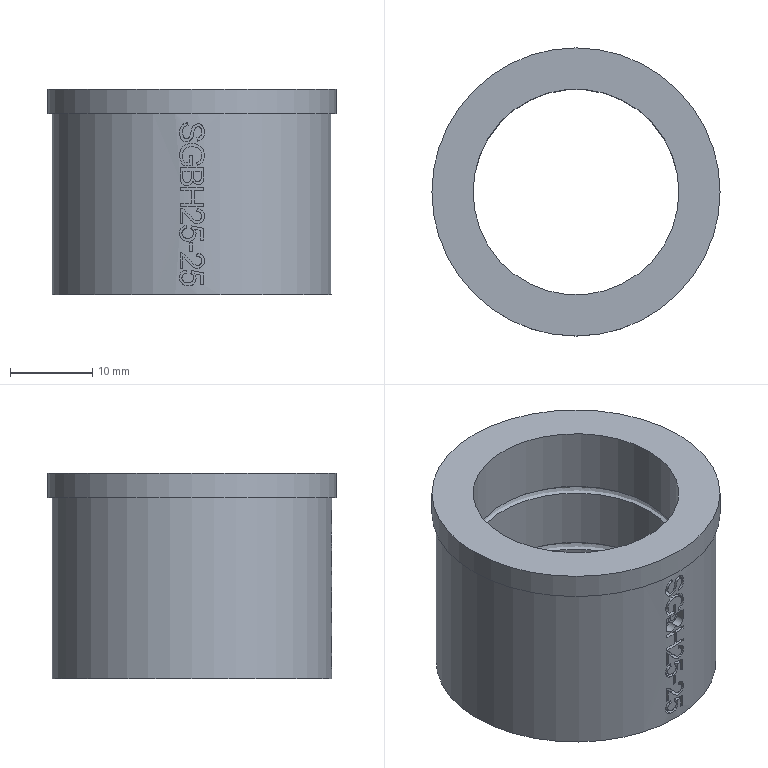Part | NX | features MI_SGBH_0851 2 | 1 solid | 142 faces | box 35 x 35 x 25 mm | volume 10500 mm3 | plane 81 | cylinder 59 | spline 2 | commonest cylinder face diameters 31.8 x9 25 x3 1.116 x2 1.174 x2 1.24 x2 1.635 x2